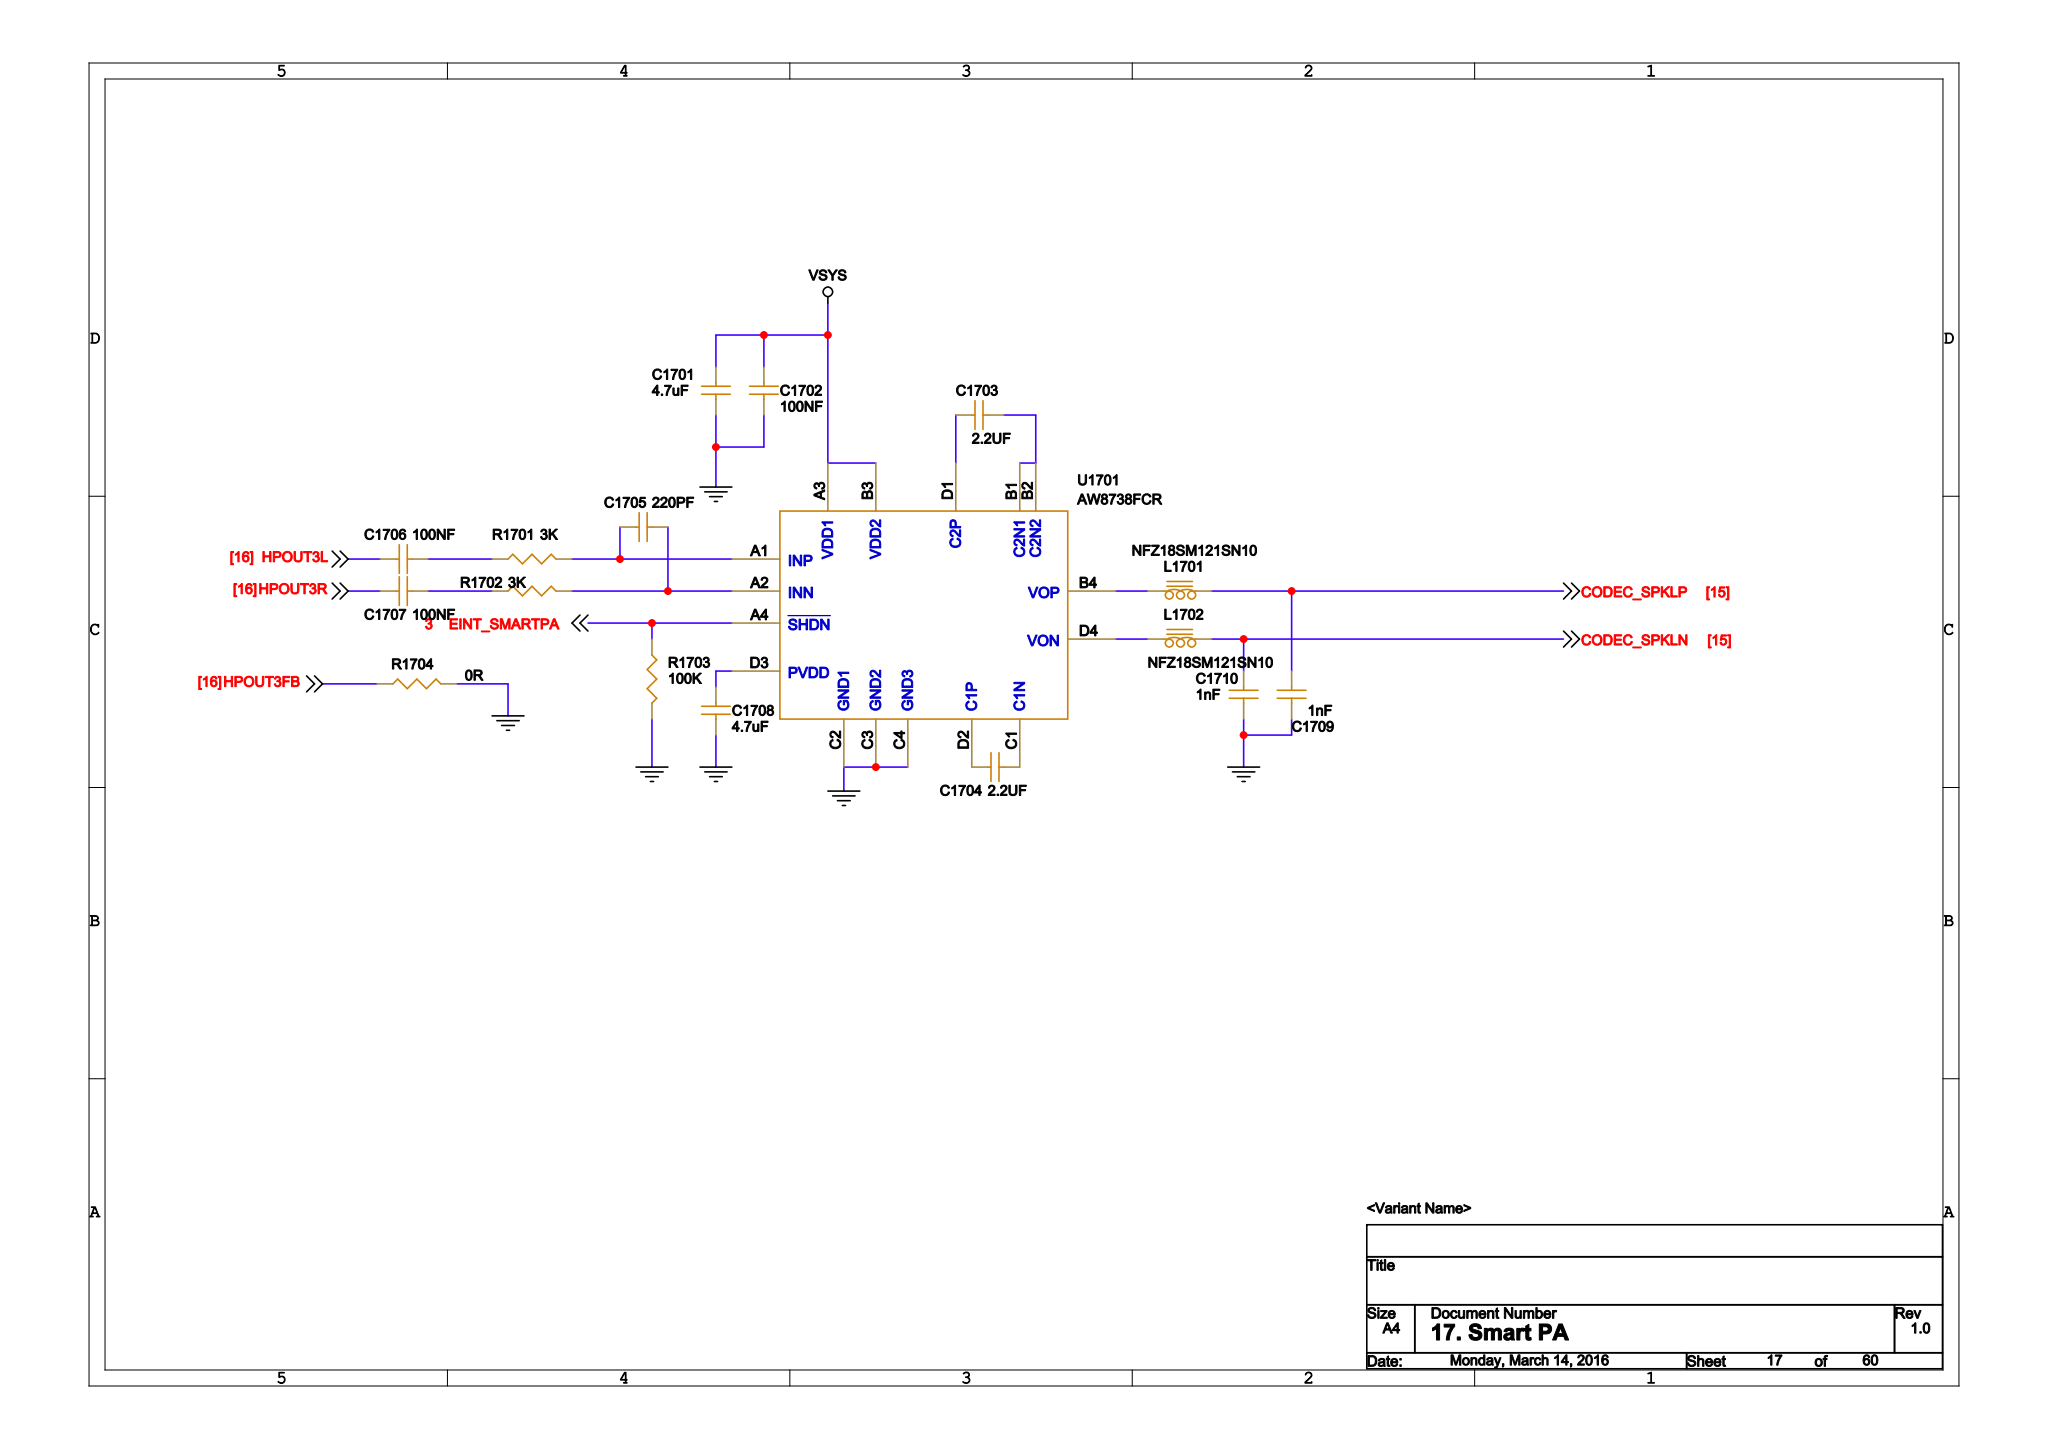Circuit board | Cadence Allegro | 1088 parts | 793 nets | one sheet of the schematic
Parts on this sheet (reference | value | footprint):
C1701 | 4.7uF | 0402-BIG
C1702 | 100NF | C0201
C1703 | 2.2UF | 0402-BIG
C1704 | 2.2UF | 0402-BIG
C1705 | 220PF | C0201
C1706 | 100NF | C0201
C1707 | 100NF | C0201
C1708 | 4.7uF | 0402-BIG
C1709 | 1nF | C0201
C1710 | 1nF | C0201
L1701 | NFZ18SM121SN10 | BLM18EG221SN1
L1702 | NFZ18SM121SN10 | BLM18EG221SN1
R1701 | 3K | R0201
R1702 | 3K | R0201
R1703 | 100K | R0201
R1704 | 0R | R0201
U1701 | AW8738FCR | FC16_2X2X0P9_0P4
Nets of these parts (net: part-pin ...):
GND: C1701-2 C1702-2 C1708-2 C1709-2 C1710-2 R1703-2 R1704-2 U1701-C2 U1701-C3 U1701-C4
VSYS: C1701-1 C1702-1 U1701-A3 U1701-B3
EINT_SMARTPA: R1703-1 U1701-A4
N344467620: C1704-2 U1701-C1
N344467621: C1704-1 U1701-D2
N34446898: C1703-2 U1701-B1 U1701-B2
N34446896: C1703-1 U1701-D1
N34446854: C1705-1 R1701-2 U1701-A1
N34446856: C1705-2 R1702-2 U1701-A2
N34446880: C1708-1 U1701-D3
N34446713: L1701-1 U1701-B4
N34446717: L1702-1 U1701-D4
HPOUT3FB: R1704-1
HPOUT3L: C1706-1
HPOUT3R: C1707-1
CODEC_SPKLP: C1709-1 L1701-2
CODEC_SPKLN: C1710-1 L1702-2
N34446874: C1706-2 R1701-1
N34446876: C1707-2 R1702-1